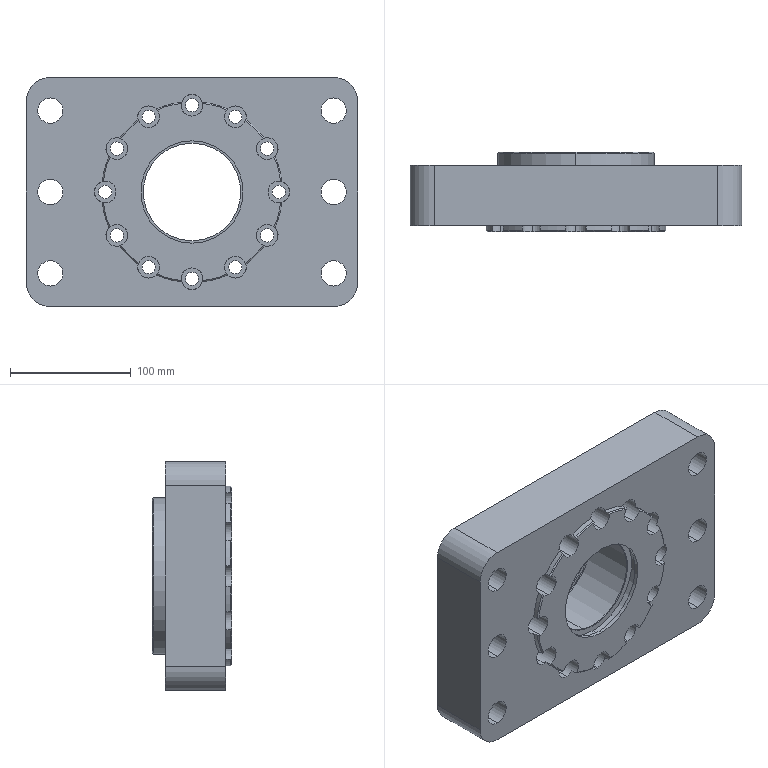Part | SolidWorks | features ICE 12, HoleWzd 3, Chamfer 2, CirPattern 2, MoveFace 2, Extrusion 1, Fillet 1 | 1 solid | 129 faces | box 275 x 66 x 190 mm | volume 2101725 mm3 | cylinder 90 | plane 25 | cone 14 | commonest cylinder face diameters 11 x24 18 x24 21 x12 150 x12 40 x4 81 x2